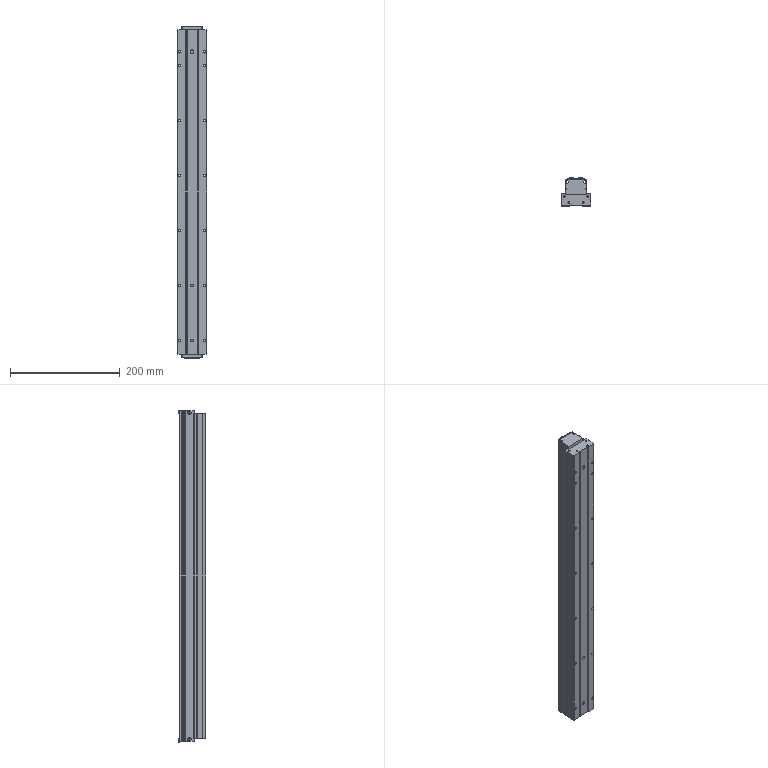Part | SolidWorks | features BaseBody 1 | 1 solid | 332 faces | box 54 x 50 x 604 mm | volume 1228026 mm3 | plane 160 | cylinder 140 | spline 16 | cone 16 | commonest cylinder face diameters 1 x29 4.4 x28 3.3 x16 6.7 x16 0.4 x14 3.1 x8